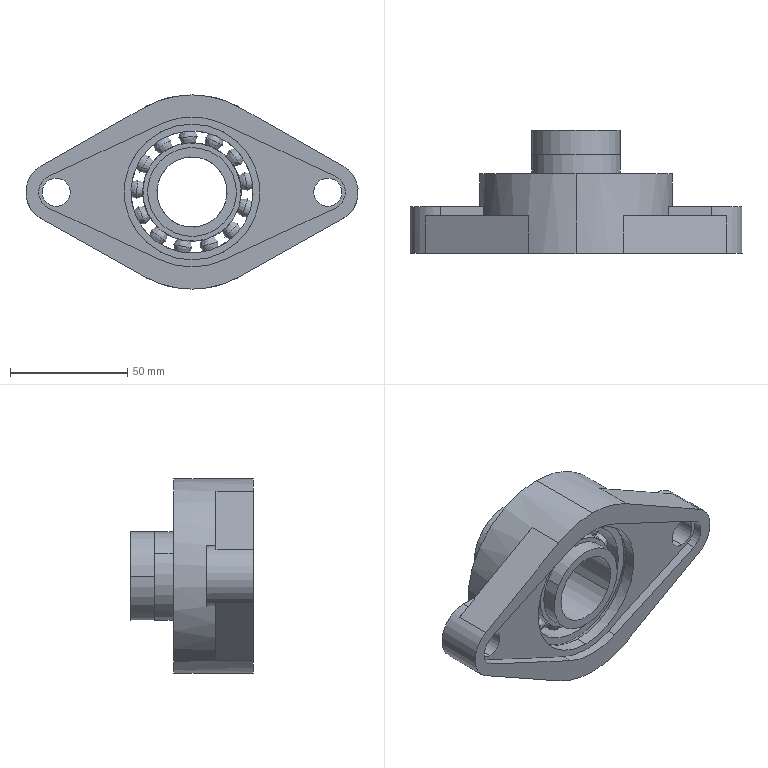Part | SolidWorks | features LayoutProfileFeature 1 | 3 solids | 90 faces | box 142 x 52.5 x 83 mm | volume 159405 mm3 | cylinder 31 | spline 30 | plane 29 | commonest cylinder face diameters 38 x6 12 x4 30 x4 58 x4 64 x3 15 x2